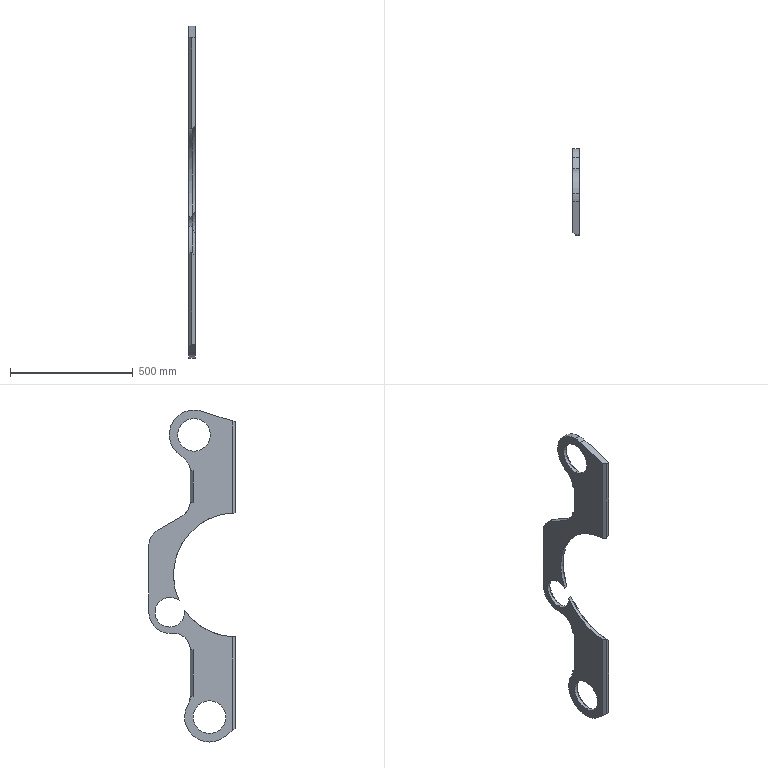Part | SolidWorks | features ICE 3, Chamfer 2, Extrusion 1, Fillet 1 | 1 solid | 46 faces | box 25 x 352.3 x 1354 mm | volume 4602346 mm3 | cylinder 19 | plane 18 | cone 9 | commonest cylinder face diameters 140 x6 133 x4 121 x3 203 x3 506 x2 171 x1
STEP:
#1=CARTESIAN_POINT('',(0.5,169.,637.5));
#2=VERTEX_POINT('',#1);
#3=CARTESIAN_POINT('',(0.5,169.,504.5));
#4=VERTEX_POINT('',#3);
#5=CARTESIAN_POINT('',(0.5,169.,571.));
#6=DIRECTION('',(1.,0.,0.));
#7=DIRECTION('',(0.,0.,-1.));
#8=AXIS2_PLACEMENT_3D('',#5,#6,#7);
#9=CIRCLE('',#8,66.5);
#10=EDGE_CURVE('',#2,#4,#9,.T.);
#11=ORIENTED_EDGE('',*,*,#10,.F.);
#12=CARTESIAN_POINT('',(12.5,169.,649.5));
#13=VERTEX_POINT('',#12);
#14=CARTESIAN_POINT('',(0.5,169.,637.5));
#15=DIRECTION('',(0.7071,0.,0.7071));
#16=VECTOR('',#15,1000.);
#17=LINE('',#14,#16);
#18=EDGE_CURVE('',#2,#13,#17,.T.);
#19=ORIENTED_EDGE('',*,*,#18,.T.);
#20=CARTESIAN_POINT('',(12.5,169.,492.5));
#21=VERTEX_POINT('',#20);
#22=CARTESIAN_POINT('',(12.5,169.,571.));
#23=DIRECTION('',(-1.,0.,0.));
#24=DIRECTION('',(0.,0.,-1.));
#25=AXIS2_PLACEMENT_3D('',#22,#23,#24);
#26=CIRCLE('',#25,78.5);
#27=EDGE_CURVE('',#21,#13,#26,.T.);
#28=ORIENTED_EDGE('',*,*,#27,.F.);
#29=CARTESIAN_POINT('',(0.5,169.,504.5));
#30=DIRECTION('',(0.7071,0.,-0.7071));
#31=VECTOR('',#30,1000.);
#32=LINE('',#29,#31);
#33=EDGE_CURVE('',#4,#21,#32,.T.);
#34=ORIENTED_EDGE('',*,*,#33,.F.);
#35=EDGE_LOOP('',(#11,#19,#28,#34));
#36=FACE_OUTER_BOUND('',#35,.T.);
#37=CARTESIAN_POINT('',(0.5,169.,571.));
#38=DIRECTION('',(1.,0.,0.));
#39=DIRECTION('',(0.,0.,-1.));
#40=AXIS2_PLACEMENT_3D('',#37,#38,#39);
#41=CONICAL_SURFACE('',#40,66.5,0.7854);
#42=ADVANCED_FACE('',(#36),#41,.F.);
#43=CARTESIAN_POINT('',(0.5,268.,-91.9));
#44=VERTEX_POINT('',#43);
#45=CARTESIAN_POINT('',(0.5,230.055,-105.278));
#46=VERTEX_POINT('',#45);
#47=CARTESIAN_POINT('',(0.5,268.,-152.4));
#48=DIRECTION('',(1.,0.,0.));
#49=DIRECTION('',(0.,0.,-1.));
#50=AXIS2_PLACEMENT_3D('',#47,#48,#49);
#51=CIRCLE('',#50,60.5);
#52=EDGE_CURVE('',#44,#46,#51,.T.);
#53=ORIENTED_EDGE('',*,*,#52,.F.);
#54=CARTESIAN_POINT('',(12.5,268.,-79.9));
#55=VERTEX_POINT('',#54);
#56=CARTESIAN_POINT('',(0.5,268.,-91.9));
#57=DIRECTION('',(0.7071,0.,0.7071));
#58=VECTOR('',#57,1000.);
#59=LINE('',#56,#58);
#60=EDGE_CURVE('',#44,#55,#59,.T.);
#61=ORIENTED_EDGE('',*,*,#60,.T.);
#62=CARTESIAN_POINT('',(12.5,252.103,-81.664));
#63=VERTEX_POINT('',#62);
#64=CARTESIAN_POINT('',(12.5,268.,-152.4));
#65=DIRECTION('',(-1.,0.,0.));
#66=DIRECTION('',(0.,0.,-1.));
#67=AXIS2_PLACEMENT_3D('',#64,#65,#66);
#68=CIRCLE('',#67,72.5);
#69=EDGE_CURVE('',#63,#55,#68,.T.);
#70=ORIENTED_EDGE('',*,*,#69,.F.);
#71=CARTESIAN_POINT('',(0.5,230.055,-105.278));
#72=CARTESIAN_POINT('',(1.802,233.534,-100.805));
#73=CARTESIAN_POINT('',(3.525,237.131,-96.657));
#74=CARTESIAN_POINT('',(7.589,244.498,-88.834));
#75=CARTESIAN_POINT('',(9.93,248.268,-85.161));
#76=CARTESIAN_POINT('',(12.5,252.103,-81.664));
#77=B_SPLINE_CURVE_WITH_KNOTS('',3,(#71,#72,#73,#74,#75,#76),.UNSPECIFIED.,.F.,.F.,(4,2,4),(0.,0.01723,0.03446),.UNSPECIFIED.);
#78=EDGE_CURVE('',#46,#63,#77,.T.);
#79=ORIENTED_EDGE('',*,*,#78,.F.);
#80=EDGE_LOOP('',(#53,#61,#70,#79));
#81=FACE_OUTER_BOUND('',#80,.T.);
#82=CARTESIAN_POINT('',(0.5,268.,-152.4));
#83=DIRECTION('',(1.,0.,0.));
#84=DIRECTION('',(0.,0.,-1.));
#85=AXIS2_PLACEMENT_3D('',#82,#83,#84);
#86=CONICAL_SURFACE('',#85,60.5,0.7854);
#87=ADVANCED_FACE('',(#81),#86,.F.);
#88=ORIENTED_EDGE('',*,*,#60,.F.);
#89=CARTESIAN_POINT('',(0.5,268.,-212.9));
#90=VERTEX_POINT('',#89);
#91=CARTESIAN_POINT('',(0.5,268.,-152.4));
#92=DIRECTION('',(1.,0.,0.));
#93=DIRECTION('',(0.,0.,-1.));
#94=AXIS2_PLACEMENT_3D('',#91,#92,#93);
#95=CIRCLE('',#94,60.5);
#96=EDGE_CURVE('',#90,#44,#95,.T.);
#97=ORIENTED_EDGE('',*,*,#96,.F.);
#98=CARTESIAN_POINT('',(12.5,268.,-224.9));
#99=VERTEX_POINT('',#98);
#100=CARTESIAN_POINT('',(0.5,268.,-212.9));
#101=DIRECTION('',(0.7071,0.,-0.7071));
#102=VECTOR('',#101,1000.);
#103=LINE('',#100,#102);
#104=EDGE_CURVE('',#90,#99,#103,.T.);
#105=ORIENTED_EDGE('',*,*,#104,.T.);
#106=CARTESIAN_POINT('',(12.5,268.,-152.4));
#107=DIRECTION('',(-1.,0.,0.));
#108=DIRECTION('',(0.,0.,-1.));
#109=AXIS2_PLACEMENT_3D('',#106,#107,#108);
#110=CIRCLE('',#109,72.5);
#111=EDGE_CURVE('',#55,#99,#110,.T.);
#112=ORIENTED_EDGE('',*,*,#111,.F.);
#113=EDGE_LOOP('',(#88,#97,#105,#112));
#114=FACE_OUTER_BOUND('',#113,.T.);
#115=CARTESIAN_POINT('',(0.5,268.,-152.4));
#116=DIRECTION('',(1.,0.,0.));
#117=DIRECTION('',(0.,0.,-1.));
#118=AXIS2_PLACEMENT_3D('',#115,#116,#117);
#119=CONICAL_SURFACE('',#118,60.5,0.7854);
#120=ADVANCED_FACE('',(#114),#119,.F.);
#121=CARTESIAN_POINT('',(0.5,106.,-513.5));
#122=VERTEX_POINT('',#121);
#123=CARTESIAN_POINT('',(0.5,106.,-646.5));
#124=VERTEX_POINT('',#123);
#125=CARTESIAN_POINT('',(0.5,106.,-580.));
#126=DIRECTION('',(1.,0.,0.));
#127=DIRECTION('',(0.,0.,-1.));
#128=AXIS2_PLACEMENT_3D('',#125,#126,#127);
#129=CIRCLE('',#128,66.5);
#130=EDGE_CURVE('',#122,#124,#129,.T.);
#131=ORIENTED_EDGE('',*,*,#130,.F.);
#132=CARTESIAN_POINT('',(12.5,106.,-501.5));
#133=VERTEX_POINT('',#132);
#134=CARTESIAN_POINT('',(0.5,106.,-513.5));
#135=DIRECTION('',(0.7071,0.,0.7071));
#136=VECTOR('',#135,1000.);
#137=LINE('',#134,#136);
#138=EDGE_CURVE('',#122,#133,#137,.T.);
#139=ORIENTED_EDGE('',*,*,#138,.T.);
#140=CARTESIAN_POINT('',(12.5,106.,-658.5));
#141=VERTEX_POINT('',#140);
#142=CARTESIAN_POINT('',(12.5,106.,-580.));
#143=DIRECTION('',(-1.,0.,0.));
#144=DIRECTION('',(0.,0.,-1.));
#145=AXIS2_PLACEMENT_3D('',#142,#143,#144);
#146=CIRCLE('',#145,78.5);
#147=EDGE_CURVE('',#141,#133,#146,.T.);
#148=ORIENTED_EDGE('',*,*,#147,.F.);
#149=CARTESIAN_POINT('',(0.5,106.,-646.5));
#150=DIRECTION('',(0.7071,0.,-0.7071));
#151=VECTOR('',#150,1000.);
#152=LINE('',#149,#151);
#153=EDGE_CURVE('',#124,#141,#152,.T.);
#154=ORIENTED_EDGE('',*,*,#153,.F.);
#155=EDGE_LOOP('',(#131,#139,#148,#154));
#156=FACE_OUTER_BOUND('',#155,.T.);
#157=CARTESIAN_POINT('',(0.5,106.,-580.));
#158=DIRECTION('',(1.,0.,0.));
#159=DIRECTION('',(0.,0.,-1.));
#160=AXIS2_PLACEMENT_3D('',#157,#158,#159);
#161=CONICAL_SURFACE('',#160,66.5,0.7854);
#162=ADVANCED_FACE('',(#156),#161,.F.);
#163=CARTESIAN_POINT('',(-12.5,106.,-513.5));
#164=VERTEX_POINT('',#163);
#165=CARTESIAN_POINT('',(-12.5,106.,-646.5));
#166=VERTEX_POINT('',#165);
#167=CARTESIAN_POINT('',(-12.5,106.,-580.));
#168=DIRECTION('',(1.,0.,0.));
#169=DIRECTION('',(0.,0.,-1.));
#170=AXIS2_PLACEMENT_3D('',#167,#168,#169);
#171=CIRCLE('',#170,66.5);
#172=EDGE_CURVE('',#164,#166,#171,.T.);
#173=ORIENTED_EDGE('',*,*,#172,.F.);
#174=CARTESIAN_POINT('',(-12.5,106.,-513.5));
#175=DIRECTION('',(1.,0.,0.));
#176=VECTOR('',#175,1000.);
#177=LINE('',#174,#176);
#178=EDGE_CURVE('',#164,#122,#177,.T.);
#179=ORIENTED_EDGE('',*,*,#178,.T.);
#180=ORIENTED_EDGE('',*,*,#130,.T.);
#181=CARTESIAN_POINT('',(-12.5,106.,-646.5));
#182=DIRECTION('',(1.,0.,0.));
#183=VECTOR('',#182,1000.);
#184=LINE('',#181,#183);
#185=EDGE_CURVE('',#166,#124,#184,.T.);
#186=ORIENTED_EDGE('',*,*,#185,.F.);
#187=EDGE_LOOP('',(#173,#179,#180,#186));
#188=FACE_OUTER_BOUND('',#187,.T.);
#189=CARTESIAN_POINT('',(-12.5,106.,-580.));
#190=DIRECTION('',(1.,0.,0.));
#191=DIRECTION('',(0.,0.,-1.));
#192=AXIS2_PLACEMENT_3D('',#189,#190,#191);
#193=CYLINDRICAL_SURFACE('',#192,66.5);
#194=ADVANCED_FACE('',(#188),#193,.F.);
#195=CARTESIAN_POINT('',(-12.5,169.,637.5));
#196=VERTEX_POINT('',#195);
#197=CARTESIAN_POINT('',(-12.5,169.,504.5));
#198=VERTEX_POINT('',#197);
#199=CARTESIAN_POINT('',(-12.5,169.,571.));
#200=DIRECTION('',(1.,0.,0.));
#201=DIRECTION('',(0.,0.,-1.));
#202=AXIS2_PLACEMENT_3D('',#199,#200,#201);
#203=CIRCLE('',#202,66.5);
#204=EDGE_CURVE('',#196,#198,#203,.T.);
#205=ORIENTED_EDGE('',*,*,#204,.F.);
#206=CARTESIAN_POINT('',(-12.5,169.,637.5));
#207=DIRECTION('',(1.,0.,0.));
#208=VECTOR('',#207,1000.);
#209=LINE('',#206,#208);
#210=EDGE_CURVE('',#196,#2,#209,.T.);
#211=ORIENTED_EDGE('',*,*,#210,.T.);
#212=ORIENTED_EDGE('',*,*,#10,.T.);
#213=CARTESIAN_POINT('',(-12.5,169.,504.5));
#214=DIRECTION('',(1.,0.,0.));
#215=VECTOR('',#214,1000.);
#216=LINE('',#213,#215);
#217=EDGE_CURVE('',#198,#4,#216,.T.);
#218=ORIENTED_EDGE('',*,*,#217,.F.);
#219=EDGE_LOOP('',(#205,#211,#212,#218));
#220=FACE_OUTER_BOUND('',#219,.T.);
#221=CARTESIAN_POINT('',(-12.5,169.,571.));
#222=DIRECTION('',(1.,0.,0.));
#223=DIRECTION('',(0.,0.,-1.));
#224=AXIS2_PLACEMENT_3D('',#221,#222,#223);
#225=CYLINDRICAL_SURFACE('',#224,66.5);
#226=ADVANCED_FACE('',(#220),#225,.F.);
#227=CARTESIAN_POINT('',(-12.5,268.,-91.9));
#228=VERTEX_POINT('',#227);
#229=CARTESIAN_POINT('',(-12.5,230.055,-105.278));
#230=VERTEX_POINT('',#229);
#231=CARTESIAN_POINT('',(-12.5,268.,-152.4));
#232=DIRECTION('',(1.,0.,0.));
#233=DIRECTION('',(0.,0.,-1.));
#234=AXIS2_PLACEMENT_3D('',#231,#232,#233);
#235=CIRCLE('',#234,60.5);
#236=EDGE_CURVE('',#228,#230,#235,.T.);
#237=ORIENTED_EDGE('',*,*,#236,.F.);
#238=CARTESIAN_POINT('',(-12.5,268.,-91.9));
#239=DIRECTION('',(1.,0.,0.));
#240=VECTOR('',#239,1000.);
#241=LINE('',#238,#240);
#242=EDGE_CURVE('',#228,#44,#241,.T.);
#243=ORIENTED_EDGE('',*,*,#242,.T.);
#244=ORIENTED_EDGE('',*,*,#52,.T.);
#245=CARTESIAN_POINT('',(0.,230.055,-105.278));
#246=DIRECTION('',(1.,0.,0.));
#247=VECTOR('',#246,1000.);
#248=LINE('',#245,#247);
#249=EDGE_CURVE('',#230,#46,#248,.T.);
#250=ORIENTED_EDGE('',*,*,#249,.F.);
#251=EDGE_LOOP('',(#237,#243,#244,#250));
#252=FACE_OUTER_BOUND('',#251,.T.);
#253=CARTESIAN_POINT('',(-12.5,268.,-152.4));
#254=DIRECTION('',(1.,0.,0.));
#255=DIRECTION('',(0.,0.,-1.));
#256=AXIS2_PLACEMENT_3D('',#253,#254,#255);
#257=CYLINDRICAL_SURFACE('',#256,60.5);
#258=ADVANCED_FACE('',(#252),#257,.F.);
#259=ORIENTED_EDGE('',*,*,#242,.F.);
#260=CARTESIAN_POINT('',(-12.5,268.,-212.9));
#261=VERTEX_POINT('',#260);
#262=CARTESIAN_POINT('',(-12.5,268.,-152.4));
#263=DIRECTION('',(1.,0.,0.));
#264=DIRECTION('',(0.,0.,-1.));
#265=AXIS2_PLACEMENT_3D('',#262,#263,#264);
#266=CIRCLE('',#265,60.5);
#267=EDGE_CURVE('',#261,#228,#266,.T.);
#268=ORIENTED_EDGE('',*,*,#267,.F.);
#269=CARTESIAN_POINT('',(-12.5,268.,-212.9));
#270=DIRECTION('',(1.,0.,0.));
#271=VECTOR('',#270,1000.);
#272=LINE('',#269,#271);
#273=EDGE_CURVE('',#261,#90,#272,.T.);
#274=ORIENTED_EDGE('',*,*,#273,.T.);
#275=ORIENTED_EDGE('',*,*,#96,.T.);
#276=EDGE_LOOP('',(#259,#268,#274,#275));
#277=FACE_OUTER_BOUND('',#276,.T.);
#278=CARTESIAN_POINT('',(-12.5,268.,-152.4));
#279=DIRECTION('',(1.,0.,0.));
#280=DIRECTION('',(0.,0.,-1.));
#281=AXIS2_PLACEMENT_3D('',#278,#279,#280);
#282=CYLINDRICAL_SURFACE('',#281,60.5);
#283=ADVANCED_FACE('',(#277),#282,.F.);
#284=CARTESIAN_POINT('',(12.5,254.,-237.268));
#285=VERTEX_POINT('',#284);
#286=CARTESIAN_POINT('',(12.5,260.302,-237.553));
#287=VERTEX_POINT('',#286);
#288=CARTESIAN_POINT('',(12.5,254.,-307.268));
#289=DIRECTION('',(-1.,0.,0.));
#290=DIRECTION('',(0.,0.,-1.));
#291=AXIS2_PLACEMENT_3D('',#288,#289,#290);
#292=CIRCLE('',#291,70.);
#293=EDGE_CURVE('',#285,#287,#292,.T.);
#294=ORIENTED_EDGE('',*,*,#293,.F.);
#295=CARTESIAN_POINT('',(-12.5,254.,-237.268));
#296=VERTEX_POINT('',#295);
#297=CARTESIAN_POINT('',(12.5,254.,-237.268));
#298=DIRECTION('',(-1.,0.,0.));
#299=VECTOR('',#298,1000.);
#300=LINE('',#297,#299);
#301=EDGE_CURVE('',#285,#296,#300,.T.);
#302=ORIENTED_EDGE('',*,*,#301,.T.);
#303=CARTESIAN_POINT('',(-12.5,260.302,-237.553));
#304=VERTEX_POINT('',#303);
#305=CARTESIAN_POINT('',(-12.5,254.,-307.268));
#306=DIRECTION('',(-1.,0.,0.));
#307=DIRECTION('',(0.,0.,-1.));
#308=AXIS2_PLACEMENT_3D('',#305,#306,#307);
#309=CIRCLE('',#308,70.);
#310=EDGE_CURVE('',#296,#304,#309,.T.);
#311=ORIENTED_EDGE('',*,*,#310,.T.);
#312=CARTESIAN_POINT('',(12.5,260.302,-237.553));
#313=DIRECTION('',(-1.,0.,0.));
#314=VECTOR('',#313,1000.);
#315=LINE('',#312,#314);
#316=EDGE_CURVE('',#287,#304,#315,.T.);
#317=ORIENTED_EDGE('',*,*,#316,.F.);
#318=EDGE_LOOP('',(#294,#302,#311,#317));
#319=FACE_OUTER_BOUND('',#318,.T.);
#320=CARTESIAN_POINT('',(12.5,254.,-307.268));
#321=DIRECTION('',(-1.,0.,0.));
#322=DIRECTION('',(0.,0.,1.));
#323=AXIS2_PLACEMENT_3D('',#320,#321,#322);
#324=CYLINDRICAL_SURFACE('',#323,70.);
#325=ADVANCED_FACE('',(#319),#324,.F.);
#326=CARTESIAN_POINT('',(12.5,169.,672.5));
#327=VERTEX_POINT('',#326);
#328=CARTESIAN_POINT('',(12.5,138.146,667.697));
#329=VERTEX_POINT('',#328);
#330=CARTESIAN_POINT('',(12.5,169.,571.));
#331=DIRECTION('',(1.,0.,0.));
#332=DIRECTION('',(0.,0.,-1.));
#333=AXIS2_PLACEMENT_3D('',#330,#331,#332);
#334=CIRCLE('',#333,101.5);
#335=EDGE_CURVE('',#327,#329,#334,.T.);
#336=ORIENTED_EDGE('',*,*,#335,.F.);
#337=CARTESIAN_POINT('',(-12.5,169.,672.5));
#338=VERTEX_POINT('',#337);
#339=CARTESIAN_POINT('',(12.5,169.,672.5));
#340=DIRECTION('',(-1.,0.,0.));
#341=VECTOR('',#340,1000.);
#342=LINE('',#339,#341);
#343=EDGE_CURVE('',#327,#338,#342,.T.);
#344=ORIENTED_EDGE('',*,*,#343,.T.);
#345=CARTESIAN_POINT('',(-12.5,138.146,667.697));
#346=VERTEX_POINT('',#345);
#347=CARTESIAN_POINT('',(-12.5,169.,571.));
#348=DIRECTION('',(1.,0.,0.));
#349=DIRECTION('',(0.,0.,-1.));
#350=AXIS2_PLACEMENT_3D('',#347,#348,#349);
#351=CIRCLE('',#350,101.5);
#352=EDGE_CURVE('',#338,#346,#351,.T.);
#353=ORIENTED_EDGE('',*,*,#352,.T.);
#354=CARTESIAN_POINT('',(12.5,138.146,667.697));
#355=DIRECTION('',(-1.,0.,0.));
#356=VECTOR('',#355,1000.);
#357=LINE('',#354,#356);
#358=EDGE_CURVE('',#329,#346,#357,.T.);
#359=ORIENTED_EDGE('',*,*,#358,.F.);
#360=EDGE_LOOP('',(#336,#344,#353,#359));
#361=FACE_OUTER_BOUND('',#360,.T.);
#362=CARTESIAN_POINT('',(12.5,169.,571.));
#363=DIRECTION('',(-1.,0.,0.));
#364=DIRECTION('',(0.,0.,1.));
#365=AXIS2_PLACEMENT_3D('',#362,#363,#364);
#366=CYLINDRICAL_SURFACE('',#365,101.5);
#367=ADVANCED_FACE('',(#361),#366,.T.);
#368=CARTESIAN_POINT('',(-12.5,106.,-580.));
#369=DIRECTION('',(1.,0.,0.));
#370=DIRECTION('',(0.,0.,-1.));
#371=AXIS2_PLACEMENT_3D('',#368,#369,#370);
#372=CIRCLE('',#371,66.5);
#373=EDGE_CURVE('',#166,#164,#372,.T.);
#374=ORIENTED_EDGE('',*,*,#373,.T.);
#375=ORIENTED_EDGE('',*,*,#172,.T.);
#376=EDGE_LOOP('',(#374,#375));
#377=FACE_BOUND('',#376,.T.);
#378=CARTESIAN_POINT('',(-12.5,169.,571.));
#379=DIRECTION('',(1.,0.,0.));
#380=DIRECTION('',(0.,0.,-1.));
#381=AXIS2_PLACEMENT_3D('',#378,#379,#380);
#382=CIRCLE('',#381,66.5);
#383=EDGE_CURVE('',#198,#196,#382,.T.);
#384=ORIENTED_EDGE('',*,*,#383,.T.);
#385=ORIENTED_EDGE('',*,*,#204,.T.);
#386=EDGE_LOOP('',(#384,#385));
#387=FACE_BOUND('',#386,.T.);
#388=CARTESIAN_POINT('',(-12.5,184.019,-495.));
#389=VERTEX_POINT('',#388);
#390=CARTESIAN_POINT('',(-12.5,172.,-495.));
#391=VERTEX_POINT('',#390);
#392=CARTESIAN_POINT('',(-12.5,190.,-495.));
#393=DIRECTION('',(0.,-1.,0.));
#394=VECTOR('',#393,1000.);
#395=LINE('',#392,#394);
#396=EDGE_CURVE('',#389,#391,#395,.T.);
#397=ORIENTED_EDGE('',*,*,#396,.F.);
#398=CARTESIAN_POINT('',(-12.5,193.592,-528.717));
#399=VERTEX_POINT('',#398);
#400=CARTESIAN_POINT('',(-12.5,254.,-493.35));
#401=DIRECTION('',(1.,0.,0.));
#402=DIRECTION('',(0.,0.,-1.));
#403=AXIS2_PLACEMENT_3D('',#400,#401,#402);
#404=CIRCLE('',#403,70.);
#405=EDGE_CURVE('',#389,#399,#404,.T.);
#406=ORIENTED_EDGE('',*,*,#405,.T.);
#407=CARTESIAN_POINT('',(-12.5,40.757,-657.754));
#408=VERTEX_POINT('',#407);
#409=CARTESIAN_POINT('',(-12.5,106.,-580.));
#410=DIRECTION('',(1.,0.,0.));
#411=DIRECTION('',(0.,0.,-1.));
#412=AXIS2_PLACEMENT_3D('',#409,#410,#411);
#413=CIRCLE('',#412,101.5);
#414=EDGE_CURVE('',#408,#399,#413,.T.);
#415=ORIENTED_EDGE('',*,*,#414,.F.);
#416=CARTESIAN_POINT('',(-12.5,13.2,-634.63));
#417=VERTEX_POINT('',#416);
#418=CARTESIAN_POINT('',(-12.5,40.757,-657.754));
#419=DIRECTION('',(0.,0.766,-0.6428));
#420=VECTOR('',#419,1000.);
#421=LINE('',#418,#420);
#422=EDGE_CURVE('',#417,#408,#421,.T.);
#423=ORIENTED_EDGE('',*,*,#422,.F.);
#424=CARTESIAN_POINT('',(-12.5,13.2,-252.655));
#425=VERTEX_POINT('',#424);
#426=CARTESIAN_POINT('',(-12.5,13.2,571.));
#427=DIRECTION('',(0.,0.,1.));
#428=VECTOR('',#427,1000.);
#429=LINE('',#426,#428);
#430=EDGE_CURVE('',#417,#425,#429,.T.);
#431=ORIENTED_EDGE('',*,*,#430,.T.);
#432=CARTESIAN_POINT('',(-12.5,208.102,-143.883));
#433=VERTEX_POINT('',#432);
#434=CARTESIAN_POINT('',(-12.5,0.,0.));
#435=DIRECTION('',(-1.,0.,0.));
#436=DIRECTION('',(0.,0.,-1.));
#437=AXIS2_PLACEMENT_3D('',#434,#435,#436);
#438=CIRCLE('',#437,253.);
#439=EDGE_CURVE('',#433,#425,#438,.T.);
#440=ORIENTED_EDGE('',*,*,#439,.F.);
#441=CARTESIAN_POINT('',(-12.5,268.,-152.4));
#442=DIRECTION('',(1.,0.,0.));
#443=DIRECTION('',(0.,0.,-1.));
#444=AXIS2_PLACEMENT_3D('',#441,#442,#443);
#445=CIRCLE('',#444,60.5);
#446=EDGE_CURVE('',#433,#261,#445,.T.);
#447=ORIENTED_EDGE('',*,*,#446,.T.);
#448=ORIENTED_EDGE('',*,*,#267,.T.);
#449=ORIENTED_EDGE('',*,*,#236,.T.);
#450=CARTESIAN_POINT('',(-12.5,13.2,252.655));
#451=VERTEX_POINT('',#450);
#452=CARTESIAN_POINT('',(-12.5,0.,0.));
#453=DIRECTION('',(-1.,0.,0.));
#454=DIRECTION('',(0.,0.,-1.));
#455=AXIS2_PLACEMENT_3D('',#452,#453,#454);
#456=CIRCLE('',#455,253.);
#457=EDGE_CURVE('',#451,#230,#456,.T.);
#458=ORIENTED_EDGE('',*,*,#457,.F.);
#459=CARTESIAN_POINT('',(-12.5,13.2,627.829));
#460=VERTEX_POINT('',#459);
#461=CARTESIAN_POINT('',(-12.5,13.2,571.));
#462=DIRECTION('',(0.,0.,1.));
#463=VECTOR('',#462,1000.);
#464=LINE('',#461,#463);
#465=EDGE_CURVE('',#451,#460,#464,.T.);
#466=ORIENTED_EDGE('',*,*,#465,.T.);
#467=CARTESIAN_POINT('',(-12.5,1.2,624.));
#468=DIRECTION('',(0.,-0.9527,-0.304));
#469=VECTOR('',#468,1000.);
#470=LINE('',#467,#469);
#471=EDGE_CURVE('',#346,#460,#470,.T.);
#472=ORIENTED_EDGE('',*,*,#471,.F.);
#473=ORIENTED_EDGE('',*,*,#352,.F.);
#474=CARTESIAN_POINT('',(-12.5,219.306,482.844));
#475=VERTEX_POINT('',#474);
#476=CARTESIAN_POINT('',(-12.5,169.,571.));
#477=DIRECTION('',(1.,0.,0.));
#478=DIRECTION('',(0.,0.,-1.));
#479=AXIS2_PLACEMENT_3D('',#476,#477,#478);
#480=CIRCLE('',#479,101.5);
#481=EDGE_CURVE('',#475,#338,#480,.T.);
#482=ORIENTED_EDGE('',*,*,#481,.F.);
#483=CARTESIAN_POINT('',(-12.5,184.062,425.));
#484=VERTEX_POINT('',#483);
#485=CARTESIAN_POINT('',(-12.5,254.,422.046));
#486=DIRECTION('',(1.,0.,0.));
#487=DIRECTION('',(0.,0.,-1.));
#488=AXIS2_PLACEMENT_3D('',#485,#486,#487);
#489=CIRCLE('',#488,70.);
#490=EDGE_CURVE('',#475,#484,#489,.T.);
#491=ORIENTED_EDGE('',*,*,#490,.T.);
#492=CARTESIAN_POINT('',(-12.5,172.,425.));
#493=VERTEX_POINT('',#492);
#494=CARTESIAN_POINT('',(-12.5,172.,425.));
#495=DIRECTION('',(0.,-1.,0.));
#496=VECTOR('',#495,1000.);
#497=LINE('',#494,#496);
#498=EDGE_CURVE('',#484,#493,#497,.T.);
#499=ORIENTED_EDGE('',*,*,#498,.T.);
#500=CARTESIAN_POINT('',(-12.5,172.,295.));
#501=VERTEX_POINT('',#500);
#502=CARTESIAN_POINT('',(-12.5,172.,295.));
#503=DIRECTION('',(0.,0.,1.));
#504=VECTOR('',#503,1000.);
#505=LINE('',#502,#504);
#506=EDGE_CURVE('',#501,#493,#505,.T.);
#507=ORIENTED_EDGE('',*,*,#506,.F.);
#508=CARTESIAN_POINT('',(-12.5,184.139,295.));
#509=VERTEX_POINT('',#508);
#510=CARTESIAN_POINT('',(-12.5,172.,295.));
#511=DIRECTION('',(0.,-1.,0.));
#512=VECTOR('',#511,1000.);
#513=LINE('',#510,#512);
#514=EDGE_CURVE('',#509,#501,#513,.T.);
#515=ORIENTED_EDGE('',*,*,#514,.F.);
#516=CARTESIAN_POINT('',(-12.5,219.,238.793));
#517=VERTEX_POINT('',#516);
#518=CARTESIAN_POINT('',(-12.5,254.,299.415));
#519=DIRECTION('',(1.,0.,0.));
#520=DIRECTION('',(0.,0.,-1.));
#521=AXIS2_PLACEMENT_3D('',#518,#519,#520);
#522=CIRCLE('',#521,70.);
#523=EDGE_CURVE('',#509,#517,#522,.T.);
#524=ORIENTED_EDGE('',*,*,#523,.T.);
#525=CARTESIAN_POINT('',(-12.5,318.5,181.346));
#526=VERTEX_POINT('',#525);
#527=CARTESIAN_POINT('',(-12.5,353.5,161.139));
#528=DIRECTION('',(0.,-0.866,0.5));
#529=VECTOR('',#528,1000.);
#530=LINE('',#527,#529);
#531=EDGE_CURVE('',#526,#517,#530,.T.);
#532=ORIENTED_EDGE('',*,*,#531,.F.);
#533=CARTESIAN_POINT('',(-12.5,353.5,120.725));
#534=VERTEX_POINT('',#533);
#535=CARTESIAN_POINT('',(-12.5,283.5,120.725));
#536=DIRECTION('',(-1.,0.,0.));
#537=DIRECTION('',(0.,0.,-1.));
#538=AXIS2_PLACEMENT_3D('',#535,#536,#537);
#539=CIRCLE('',#538,70.);
#540=EDGE_CURVE('',#526,#534,#539,.T.);
#541=ORIENTED_EDGE('',*,*,#540,.T.);
#542=CARTESIAN_POINT('',(-12.5,353.5,-152.4));
#543=VERTEX_POINT('',#542);
#544=CARTESIAN_POINT('',(-12.5,353.5,161.139));
#545=DIRECTION('',(0.,0.,1.));
#546=VECTOR('',#545,1000.);
#547=LINE('',#544,#546);
#548=EDGE_CURVE('',#543,#534,#547,.T.);
#549=ORIENTED_EDGE('',*,*,#548,.F.);
#550=CARTESIAN_POINT('',(-12.5,268.,-152.4));
#551=DIRECTION('',(1.,0.,0.));
#552=DIRECTION('',(0.,0.,-1.));
#553=AXIS2_PLACEMENT_3D('',#550,#551,#552);
#554=CIRCLE('',#553,85.5);
#555=EDGE_CURVE('',#304,#543,#554,.T.);
#556=ORIENTED_EDGE('',*,*,#555,.F.);
#557=ORIENTED_EDGE('',*,*,#310,.F.);
#558=CARTESIAN_POINT('',(-12.5,184.037,-305.));
#559=VERTEX_POINT('',#558);
#560=CARTESIAN_POINT('',(-12.5,254.,-307.268));
#561=DIRECTION('',(-1.,0.,0.));
#562=DIRECTION('',(0.,0.,-1.));
#563=AXIS2_PLACEMENT_3D('',#560,#561,#562);
#564=CIRCLE('',#563,70.);
#565=EDGE_CURVE('',#559,#296,#564,.T.);
#566=ORIENTED_EDGE('',*,*,#565,.F.);
#567=CARTESIAN_POINT('',(-12.5,172.,-305.));
#568=VERTEX_POINT('',#567);
#569=CARTESIAN_POINT('',(-12.5,190.,-305.));
#570=DIRECTION('',(0.,-1.,0.));
#571=VECTOR('',#570,1000.);
#572=LINE('',#569,#571);
#573=EDGE_CURVE('',#559,#568,#572,.T.);
#574=ORIENTED_EDGE('',*,*,#573,.T.);
#575=CARTESIAN_POINT('',(-12.5,172.,-495.));
#576=DIRECTION('',(0.,0.,1.));
#577=VECTOR('',#576,1000.);
#578=LINE('',#575,#577);
#579=EDGE_CURVE('',#391,#568,#578,.T.);
#580=ORIENTED_EDGE('',*,*,#579,.F.);
#581=EDGE_LOOP('',(#397,#406,#415,#423,#431,#440,#447,#448,#449,#458,#466,#472,#473,#482,#491,#499,#507,#515,#524,#532,#541,#549,#556,#557,#566,#574,#580));
#582=FACE_OUTER_BOUND('',#581,.T.);
#583=CARTESIAN_POINT('',(-12.5,169.,571.));
#584=DIRECTION('',(1.,0.,0.));
#585=DIRECTION('',(0.,0.,-1.));
#586=AXIS2_PLACEMENT_3D('',#583,#584,#585);
#587=PLANE('',#586);
#588=ADVANCED_FACE('',(#377,#387,#582),#587,.F.);
#589=ORIENTED_EDGE('',*,*,#439,.T.);
#590=CARTESIAN_POINT('',(-0.5,1.2,-252.997));
#591=VERTEX_POINT('',#590);
#592=CARTESIAN_POINT('',(-12.5,13.2,-252.655));
#593=CARTESIAN_POINT('',(-8.503,9.203,-252.864));
#594=CARTESIAN_POINT('',(-4.502,5.202,-252.978));
#595=CARTESIAN_POINT('',(-0.5,1.2,-252.997));
#596=(BOUNDED_CURVE()B_SPLINE_CURVE(3,(#592,#593,#594,#595),.UNSPECIFIED.,.F.,.T.)B_SPLINE_CURVE_WITH_KNOTS((4,4),(1.519,1.566),.UNSPECIFIED.)CURVE()GEOMETRIC_REPRESENTATION_ITEM()RATIONAL_B_SPLINE_CURVE((1.,0.9998,0.9998,1.))REPRESENTATION_ITEM(''));
#597=EDGE_CURVE('',#425,#591,#596,.T.);
#598=ORIENTED_EDGE('',*,*,#597,.T.);
#599=CARTESIAN_POINT('',(0.5,1.2,-252.997));
#600=VERTEX_POINT('',#599);
#601=CARTESIAN_POINT('',(12.5,1.2,-252.997));
#602=DIRECTION('',(-1.,0.,0.));
#603=VECTOR('',#602,1000.);
#604=LINE('',#601,#603);
#605=EDGE_CURVE('',#600,#591,#604,.T.);
#606=ORIENTED_EDGE('',*,*,#605,.F.);
#607=CARTESIAN_POINT('',(0.5,208.102,-143.883));
#608=VERTEX_POINT('',#607);
#609=CARTESIAN_POINT('',(0.5,0.,0.));
#610=DIRECTION('',(1.,0.,0.));
#611=DIRECTION('',(0.,0.,-1.));
#612=AXIS2_PLACEMENT_3D('',#609,#610,#611);
#613=CIRCLE('',#612,253.);
#614=EDGE_CURVE('',#600,#608,#613,.T.);
#615=ORIENTED_EDGE('',*,*,#614,.T.);
#616=CARTESIAN_POINT('',(0.,208.102,-143.883));
#617=DIRECTION('',(-1.,0.,0.));
#618=VECTOR('',#617,1000.);
#619=LINE('',#616,#618);
#620=EDGE_CURVE('',#608,#433,#619,.T.);
#621=ORIENTED_EDGE('',*,*,#620,.T.);
#622=EDGE_LOOP('',(#589,#598,#606,#615,#621));
#623=FACE_OUTER_BOUND('',#622,.T.);
#624=CARTESIAN_POINT('',(12.5,0.,0.));
#625=DIRECTION('',(-1.,0.,0.));
#626=DIRECTION('',(0.,0.,1.));
#627=AXIS2_PLACEMENT_3D('',#624,#625,#626);
#628=CYLINDRICAL_SURFACE('',#627,253.);
#629=ADVANCED_FACE('',(#623),#628,.F.);
#630=ORIENTED_EDGE('',*,*,#343,.F.);
#631=CARTESIAN_POINT('',(12.5,219.306,482.844));
#632=VERTEX_POINT('',#631);
#633=CARTESIAN_POINT('',(12.5,169.,571.));
#634=DIRECTION('',(1.,0.,0.));
#635=DIRECTION('',(0.,0.,-1.));
#636=AXIS2_PLACEMENT_3D('',#633,#634,#635);
#637=CIRCLE('',#636,101.5);
#638=EDGE_CURVE('',#632,#327,#637,.T.);
#639=ORIENTED_EDGE('',*,*,#638,.F.);
#640=CARTESIAN_POINT('',(12.5,219.306,482.844));
#641=DIRECTION('',(-1.,0.,0.));
#642=VECTOR('',#641,1000.);
#643=LINE('',#640,#642);
#644=EDGE_CURVE('',#632,#475,#643,.T.);
#645=ORIENTED_EDGE('',*,*,#644,.T.);
#646=ORIENTED_EDGE('',*,*,#481,.T.);
#647=EDGE_LOOP('',(#630,#639,#645,#646));
#648=FACE_OUTER_BOUND('',#647,.T.);
#649=CARTESIAN_POINT('',(12.5,169.,571.));
#650=DIRECTION('',(-1.,0.,0.));
#651=DIRECTION('',(0.,0.,1.));
#652=AXIS2_PLACEMENT_3D('',#649,#650,#651);
#653=CYLINDRICAL_SURFACE('',#652,101.5);
#654=ADVANCED_FACE('',(#648),#653,.T.);
#655=ORIENTED_EDGE('',*,*,#471,.T.);
#656=CARTESIAN_POINT('',(-0.5,1.2,624.));
#657=VERTEX_POINT('',#656);
#658=CARTESIAN_POINT('',(-0.5,1.2,624.));
#659=DIRECTION('',(0.6898,-0.6898,-0.2201));
#660=VECTOR('',#659,1000.);
#661=LINE('',#658,#660);
#662=EDGE_CURVE('',#460,#657,#661,.T.);
#663=ORIENTED_EDGE('',*,*,#662,.T.);
#664=CARTESIAN_POINT('',(12.5,1.2,624.));
#665=VERTEX_POINT('',#664);
#666=CARTESIAN_POINT('',(12.5,1.2,624.));
#667=DIRECTION('',(-1.,0.,0.));
#668=VECTOR('',#667,1000.);
#669=LINE('',#666,#668);
#670=EDGE_CURVE('',#665,#657,#669,.T.);
#671=ORIENTED_EDGE('',*,*,#670,.F.);
#672=CARTESIAN_POINT('',(12.5,1.2,624.));
#673=DIRECTION('',(0.,-0.9527,-0.304));
#674=VECTOR('',#673,1000.);
#675=LINE('',#672,#674);
#676=EDGE_CURVE('',#329,#665,#675,.T.);
#677=ORIENTED_EDGE('',*,*,#676,.F.);
#678=ORIENTED_EDGE('',*,*,#358,.T.);
#679=EDGE_LOOP('',(#655,#663,#671,#677,#678));
#680=FACE_OUTER_BOUND('',#679,.T.);
#681=CARTESIAN_POINT('',(12.5,1.2,624.));
#682=DIRECTION('',(0.,0.304,-0.9527));
#683=DIRECTION('',(0.,0.9527,0.304));
#684=AXIS2_PLACEMENT_3D('',#681,#682,#683);
#685=PLANE('',#684);
#686=ADVANCED_FACE('',(#680),#685,.F.);
#687=ORIENTED_EDGE('',*,*,#670,.T.);
#688=CARTESIAN_POINT('',(-0.5,1.2,252.997));
#689=VERTEX_POINT('',#688);
#690=CARTESIAN_POINT('',(-0.5,1.2,624.));
#691=DIRECTION('',(0.,0.,-1.));
#692=VECTOR('',#691,1000.);
#693=LINE('',#690,#692);
#694=EDGE_CURVE('',#657,#689,#693,.T.);
#695=ORIENTED_EDGE('',*,*,#694,.T.);
#696=CARTESIAN_POINT('',(0.5,1.2,252.997));
#697=VERTEX_POINT('',#696);
#698=CARTESIAN_POINT('',(12.5,1.2,252.997));
#699=DIRECTION('',(-1.,0.,0.));
#700=VECTOR('',#699,1000.);
#701=LINE('',#698,#700);
#702=EDGE_CURVE('',#697,#689,#701,.T.);
#703=ORIENTED_EDGE('',*,*,#702,.F.);
#704=CARTESIAN_POINT('',(12.5,1.2,264.997));
#705=VERTEX_POINT('',#704);
#706=CARTESIAN_POINT('',(0.5,1.2,252.997));
#707=CARTESIAN_POINT('',(4.5,1.2,256.997));
#708=CARTESIAN_POINT('',(8.5,1.2,260.997));
#709=CARTESIAN_POINT('',(12.5,1.2,264.997));
#710=B_SPLINE_CURVE_WITH_KNOTS('',3,(#706,#707,#708,#709),.UNSPECIFIED.,.F.,.F.,(4,4),(0.,0.01697),.UNSPECIFIED.);
#711=EDGE_CURVE('',#697,#705,#710,.T.);
#712=ORIENTED_EDGE('',*,*,#711,.T.);
#713=CARTESIAN_POINT('',(12.5,1.2,624.));
#714=DIRECTION('',(0.,0.,-1.));
#715=VECTOR('',#714,1000.);
#716=LINE('',#713,#715);
#717=EDGE_CURVE('',#665,#705,#716,.T.);
#718=ORIENTED_EDGE('',*,*,#717,.F.);
#719=EDGE_LOOP('',(#687,#695,#703,#712,#718));
#720=FACE_OUTER_BOUND('',#719,.T.);
#721=CARTESIAN_POINT('',(12.5,1.2,624.));
#722=DIRECTION('',(0.,1.,0.));
#723=DIRECTION('',(0.,0.,1.));
#724=AXIS2_PLACEMENT_3D('',#721,#722,#723);
#725=PLANE('',#724);
#726=ADVANCED_FACE('',(#720),#725,.F.);
#727=ORIENTED_EDGE('',*,*,#702,.T.);
#728=CARTESIAN_POINT('',(-0.5,1.2,252.997));
#729=CARTESIAN_POINT('',(-4.502,5.202,252.978));
#730=CARTESIAN_POINT('',(-8.503,9.203,252.864));
#731=CARTESIAN_POINT('',(-12.5,13.2,252.655));
#732=(BOUNDED_CURVE()B_SPLINE_CURVE(3,(#728,#729,#730,#731),.UNSPECIFIED.,.F.,.F.)B_SPLINE_CURVE_WITH_KNOTS((4,4),(4.717,4.765),.UNSPECIFIED.)CURVE()GEOMETRIC_REPRESENTATION_ITEM()RATIONAL_B_SPLINE_CURVE((1.,0.9998,0.9998,1.))REPRESENTATION_ITEM(''));
#733=EDGE_CURVE('',#689,#451,#732,.T.);
#734=ORIENTED_EDGE('',*,*,#733,.T.);
#735=ORIENTED_EDGE('',*,*,#457,.T.);
#736=ORIENTED_EDGE('',*,*,#249,.T.);
#737=CARTESIAN_POINT('',(0.5,0.,0.));
#738=DIRECTION('',(1.,0.,0.));
#739=DIRECTION('',(0.,0.,-1.));
#740=AXIS2_PLACEMENT_3D('',#737,#738,#739);
#741=CIRCLE('',#740,253.);
#742=EDGE_CURVE('',#46,#697,#741,.T.);
#743=ORIENTED_EDGE('',*,*,#742,.T.);
#744=EDGE_LOOP('',(#727,#734,#735,#736,#743));
#745=FACE_OUTER_BOUND('',#744,.T.);
#746=CARTESIAN_POINT('',(12.5,0.,0.));
#747=DIRECTION('',(-1.,0.,0.));
#748=DIRECTION('',(0.,0.,1.));
#749=AXIS2_PLACEMENT_3D('',#746,#747,#748);
#750=CYLINDRICAL_SURFACE('',#749,253.);
#751=ADVANCED_FACE('',(#745),#750,.F.);
#752=ORIENTED_EDGE('',*,*,#605,.T.);
#753=CARTESIAN_POINT('',(-0.5,1.2,-624.561));
#754=VERTEX_POINT('',#753);
#755=CARTESIAN_POINT('',(-0.5,1.2,-624.561));
#756=DIRECTION('',(0.,0.,-1.));
#757=VECTOR('',#756,1000.);
#758=LINE('',#755,#757);
#759=EDGE_CURVE('',#591,#754,#758,.T.);
#760=ORIENTED_EDGE('',*,*,#759,.T.);
#761=CARTESIAN_POINT('',(12.5,1.2,-624.561));
#762=VERTEX_POINT('',#761);
#763=CARTESIAN_POINT('',(12.5,1.2,-624.561));
#764=DIRECTION('',(-1.,0.,0.));
#765=VECTOR('',#764,1000.);
#766=LINE('',#763,#765);
#767=EDGE_CURVE('',#762,#754,#766,.T.);
#768=ORIENTED_EDGE('',*,*,#767,.F.);
#769=CARTESIAN_POINT('',(12.5,1.2,-264.997));
#770=VERTEX_POINT('',#769);
#771=CARTESIAN_POINT('',(12.5,1.2,-624.561));
#772=DIRECTION('',(0.,0.,-1.));
#773=VECTOR('',#772,1000.);
#774=LINE('',#771,#773);
#775=EDGE_CURVE('',#770,#762,#774,.T.);
#776=ORIENTED_EDGE('',*,*,#775,.F.);
#777=CARTESIAN_POINT('',(12.5,1.2,-264.997));
#778=CARTESIAN_POINT('',(8.5,1.2,-260.997));
#779=CARTESIAN_POINT('',(4.5,1.2,-256.997));
#780=CARTESIAN_POINT('',(0.5,1.2,-252.997));
#781=B_SPLINE_CURVE_WITH_KNOTS('',3,(#777,#778,#779,#780),.UNSPECIFIED.,.F.,.F.,(4,4),(0.,0.01697),.UNSPECIFIED.);
#782=EDGE_CURVE('',#770,#600,#781,.T.);
#783=ORIENTED_EDGE('',*,*,#782,.T.);
#784=EDGE_LOOP('',(#752,#760,#768,#776,#783));
#785=FACE_OUTER_BOUND('',#784,.T.);
#786=CARTESIAN_POINT('',(12.5,1.2,-624.561));
#787=DIRECTION('',(0.,1.,0.));
#788=DIRECTION('',(0.,0.,1.));
#789=AXIS2_PLACEMENT_3D('',#786,#787,#788);
#790=PLANE('',#789);
#791=ADVANCED_FACE('',(#785),#790,.F.);
#792=ORIENTED_EDGE('',*,*,#767,.T.);
#793=CARTESIAN_POINT('',(-0.5,1.2,-624.561));
#794=DIRECTION('',(-0.6081,0.6081,-0.5103));
#795=VECTOR('',#794,1000.);
#796=LINE('',#793,#795);
#797=EDGE_CURVE('',#754,#417,#796,.T.);
#798=ORIENTED_EDGE('',*,*,#797,.T.);
#799=ORIENTED_EDGE('',*,*,#422,.T.);
#800=CARTESIAN_POINT('',(12.5,40.757,-657.754));
#801=VERTEX_POINT('',#800);
#802=CARTESIAN_POINT('',(12.5,40.757,-657.754));
#803=DIRECTION('',(-1.,0.,0.));
#804=VECTOR('',#803,1000.);
#805=LINE('',#802,#804);
#806=EDGE_CURVE('',#801,#408,#805,.T.);
#807=ORIENTED_EDGE('',*,*,#806,.F.);
#808=CARTESIAN_POINT('',(12.5,40.757,-657.754));
#809=DIRECTION('',(0.,0.766,-0.6428));
#810=VECTOR('',#809,1000.);
#811=LINE('',#808,#810);
#812=EDGE_CURVE('',#762,#801,#811,.T.);
#813=ORIENTED_EDGE('',*,*,#812,.F.);
#814=EDGE_LOOP('',(#792,#798,#799,#807,#813));
#815=FACE_OUTER_BOUND('',#814,.T.);
#816=CARTESIAN_POINT('',(12.5,40.757,-657.754));
#817=DIRECTION('',(0.,0.6428,0.766));
#818=DIRECTION('',(0.,-0.766,0.6428));
#819=AXIS2_PLACEMENT_3D('',#816,#817,#818);
#820=PLANE('',#819);
#821=ADVANCED_FACE('',(#815),#820,.F.);
#822=ORIENTED_EDGE('',*,*,#414,.T.);
#823=CARTESIAN_POINT('',(12.5,193.592,-528.717));
#824=VERTEX_POINT('',#823);
#825=CARTESIAN_POINT('',(12.5,193.592,-528.717));
#826=DIRECTION('',(1.,0.,0.));
#827=VECTOR('',#826,1000.);
#828=LINE('',#825,#827);
#829=EDGE_CURVE('',#399,#824,#828,.T.);
#830=ORIENTED_EDGE('',*,*,#829,.T.);
#831=CARTESIAN_POINT('',(12.5,106.,-580.));
#832=DIRECTION('',(1.,0.,0.));
#833=DIRECTION('',(0.,0.,-1.));
#834=AXIS2_PLACEMENT_3D('',#831,#832,#833);
#835=CIRCLE('',#834,101.5);
#836=EDGE_CURVE('',#801,#824,#835,.T.);
#837=ORIENTED_EDGE('',*,*,#836,.F.);
#838=ORIENTED_EDGE('',*,*,#806,.T.);
#839=EDGE_LOOP('',(#822,#830,#837,#838));
#840=FACE_OUTER_BOUND('',#839,.T.);
#841=CARTESIAN_POINT('',(12.5,106.,-580.));
#842=DIRECTION('',(-1.,0.,0.));
#843=DIRECTION('',(0.,0.,1.));
#844=AXIS2_PLACEMENT_3D('',#841,#842,#843);
#845=CYLINDRICAL_SURFACE('',#844,101.5);
#846=ADVANCED_FACE('',(#840),#845,.T.);
#847=CARTESIAN_POINT('',(12.5,184.,-493.35));
#848=VERTEX_POINT('',#847);
#849=CARTESIAN_POINT('',(-0.5,184.,-493.35));
#850=VERTEX_POINT('',#849);
#851=CARTESIAN_POINT('',(-12.5,184.,-493.35));
#852=DIRECTION('',(-1.,0.,0.));
#853=VECTOR('',#852,1000.);
#854=LINE('',#851,#853);
#855=EDGE_CURVE('',#848,#850,#854,.T.);
#856=ORIENTED_EDGE('',*,*,#855,.T.);
#857=CARTESIAN_POINT('',(-0.5,184.,-307.268));
#858=VERTEX_POINT('',#857);
#859=CARTESIAN_POINT('',(-0.5,184.,-307.268));
#860=DIRECTION('',(0.,0.,1.));
#861=VECTOR('',#860,1000.);
#862=LINE('',#859,#861);
#863=EDGE_CURVE('',#850,#858,#862,.T.);
#864=ORIENTED_EDGE('',*,*,#863,.T.);
#865=CARTESIAN_POINT('',(12.5,184.,-307.268));
#866=VERTEX_POINT('',#865);
#867=CARTESIAN_POINT('',(12.5,184.,-307.268));
#868=DIRECTION('',(-1.,0.,0.));
#869=VECTOR('',#868,1000.);
#870=LINE('',#867,#869);
#871=EDGE_CURVE('',#866,#858,#870,.T.);
#872=ORIENTED_EDGE('',*,*,#871,.F.);
#873=CARTESIAN_POINT('',(12.5,184.,-307.268));
#874=DIRECTION('',(0.,0.,1.));
#875=VECTOR('',#874,1000.);
#876=LINE('',#873,#875);
#877=EDGE_CURVE('',#848,#866,#876,.T.);
#878=ORIENTED_EDGE('',*,*,#877,.F.);
#879=EDGE_LOOP('',(#856,#864,#872,#878));
#880=FACE_OUTER_BOUND('',#879,.T.);
#881=CARTESIAN_POINT('',(12.5,184.,-307.268));
#882=DIRECTION('',(0.,-1.,0.));
#883=DIRECTION('',(0.,0.,-1.));
#884=AXIS2_PLACEMENT_3D('',#881,#882,#883);
#885=PLANE('',#884);
#886=ADVANCED_FACE('',(#880),#885,.F.);
#887=ORIENTED_EDGE('',*,*,#301,.F.);
#888=CARTESIAN_POINT('',(12.5,254.,-307.268));
#889=DIRECTION('',(-1.,0.,0.));
#890=DIRECTION('',(0.,0.,-1.));
#891=AXIS2_PLACEMENT_3D('',#888,#889,#890);
#892=CIRCLE('',#891,70.);
#893=EDGE_CURVE('',#866,#285,#892,.T.);
#894=ORIENTED_EDGE('',*,*,#893,.F.);
#895=ORIENTED_EDGE('',*,*,#871,.T.);
#896=CARTESIAN_POINT('',(-0.4632,184.037,-305.));
#897=VERTEX_POINT('',#896);
#898=CARTESIAN_POINT('',(-0.5,184.,-307.268));
#899=CARTESIAN_POINT('',(-0.5,184.,-306.512));
#900=CARTESIAN_POINT('',(-0.4877,184.012,-305.756));
#901=CARTESIAN_POINT('',(-0.4632,184.037,-305.));
#902=(BOUNDED_CURVE()B_SPLINE_CURVE(3,(#898,#899,#900,#901),.UNSPECIFIED.,.F.,.T.)B_SPLINE_CURVE_WITH_KNOTS((4,4),(0.,0.03241),.UNSPECIFIED.)CURVE()GEOMETRIC_REPRESENTATION_ITEM()RATIONAL_B_SPLINE_CURVE((1.,0.9999,0.9999,1.))REPRESENTATION_ITEM(''));
#903=EDGE_CURVE('',#858,#897,#902,.T.);
#904=ORIENTED_EDGE('',*,*,#903,.T.);
#905=CARTESIAN_POINT('',(12.5,184.037,-305.));
#906=DIRECTION('',(-1.,0.,0.));
#907=VECTOR('',#906,1000.);
#908=LINE('',#905,#907);
#909=EDGE_CURVE('',#897,#559,#908,.T.);
#910=ORIENTED_EDGE('',*,*,#909,.T.);
#911=ORIENTED_EDGE('',*,*,#565,.T.);
#912=EDGE_LOOP('',(#887,#894,#895,#904,#910,#911));
#913=FACE_OUTER_BOUND('',#912,.T.);
#914=CARTESIAN_POINT('',(12.5,254.,-307.268));
#915=DIRECTION('',(-1.,0.,0.));
#916=DIRECTION('',(0.,0.,1.));
#917=AXIS2_PLACEMENT_3D('',#914,#915,#916);
#918=CYLINDRICAL_SURFACE('',#917,70.);
#919=ADVANCED_FACE('',(#913),#918,.F.);
#920=ORIENTED_EDGE('',*,*,#555,.T.);
#921=CARTESIAN_POINT('',(12.5,353.5,-152.4));
#922=VERTEX_POINT('',#921);
#923=CARTESIAN_POINT('',(12.5,353.5,-152.4));
#924=DIRECTION('',(-1.,0.,0.));
#925=VECTOR('',#924,1000.);
#926=LINE('',#923,#925);
#927=EDGE_CURVE('',#922,#543,#926,.T.);
#928=ORIENTED_EDGE('',*,*,#927,.F.);
#929=CARTESIAN_POINT('',(12.5,268.,-152.4));
#930=DIRECTION('',(1.,0.,0.));
#931=DIRECTION('',(0.,0.,-1.));
#932=AXIS2_PLACEMENT_3D('',#929,#930,#931);
#933=CIRCLE('',#932,85.5);
#934=EDGE_CURVE('',#287,#922,#933,.T.);
#935=ORIENTED_EDGE('',*,*,#934,.F.);
#936=ORIENTED_EDGE('',*,*,#316,.T.);
#937=EDGE_LOOP('',(#920,#928,#935,#936));
#938=FACE_OUTER_BOUND('',#937,.T.);
#939=CARTESIAN_POINT('',(12.5,268.,-152.4));
#940=DIRECTION('',(-1.,0.,0.));
#941=DIRECTION('',(0.,0.,1.));
#942=AXIS2_PLACEMENT_3D('',#939,#940,#941);
#943=CYLINDRICAL_SURFACE('',#942,85.5);
#944=ADVANCED_FACE('',(#938),#943,.T.);
#945=ORIENTED_EDGE('',*,*,#548,.T.);
#946=CARTESIAN_POINT('',(12.5,353.5,120.725));
#947=VERTEX_POINT('',#946);
#948=CARTESIAN_POINT('',(12.5,353.5,120.725));
#949=DIRECTION('',(1.,0.,0.));
#950=VECTOR('',#949,1000.);
#951=LINE('',#948,#950);
#952=EDGE_CURVE('',#534,#947,#951,.T.);
#953=ORIENTED_EDGE('',*,*,#952,.T.);
#954=CARTESIAN_POINT('',(12.5,353.5,161.139));
#955=DIRECTION('',(0.,0.,1.));
#956=VECTOR('',#955,1000.);
#957=LINE('',#954,#956);
#958=EDGE_CURVE('',#922,#947,#957,.T.);
#959=ORIENTED_EDGE('',*,*,#958,.F.);
#960=ORIENTED_EDGE('',*,*,#927,.T.);
#961=EDGE_LOOP('',(#945,#953,#959,#960));
#962=FACE_OUTER_BOUND('',#961,.T.);
#963=CARTESIAN_POINT('',(12.5,353.5,161.139));
#964=DIRECTION('',(0.,-1.,0.));
#965=DIRECTION('',(0.,0.,-1.));
#966=AXIS2_PLACEMENT_3D('',#963,#964,#965);
#967=PLANE('',#966);
#968=ADVANCED_FACE('',(#962),#967,.F.);
#969=CARTESIAN_POINT('',(12.5,318.5,181.346));
#970=VERTEX_POINT('',#969);
#971=CARTESIAN_POINT('',(12.5,219.,238.793));
#972=VERTEX_POINT('',#971);
#973=CARTESIAN_POINT('',(12.5,353.5,161.139));
#974=DIRECTION('',(0.,-0.866,0.5));
#975=VECTOR('',#974,1000.);
#976=LINE('',#973,#975);
#977=EDGE_CURVE('',#970,#972,#976,.T.);
#978=ORIENTED_EDGE('',*,*,#977,.F.);
#979=CARTESIAN_POINT('',(12.5,318.5,181.346));
#980=DIRECTION('',(-1.,0.,0.));
#981=VECTOR('',#980,1000.);
#982=LINE('',#979,#981);
#983=EDGE_CURVE('',#970,#526,#982,.T.);
#984=ORIENTED_EDGE('',*,*,#983,.T.);
#985=ORIENTED_EDGE('',*,*,#531,.T.);
#986=CARTESIAN_POINT('',(12.5,219.,238.793));
#987=DIRECTION('',(1.,0.,0.));
#988=VECTOR('',#987,1000.);
#989=LINE('',#986,#988);
#990=EDGE_CURVE('',#517,#972,#989,.T.);
#991=ORIENTED_EDGE('',*,*,#990,.T.);
#992=EDGE_LOOP('',(#978,#984,#985,#991));
#993=FACE_OUTER_BOUND('',#992,.T.);
#994=CARTESIAN_POINT('',(12.5,353.5,161.139));
#995=DIRECTION('',(0.,-0.5,-0.866));
#996=DIRECTION('',(0.,0.866,-0.5));
#997=AXIS2_PLACEMENT_3D('',#994,#995,#996);
#998=PLANE('',#997);
#999=ADVANCED_FACE('',(#993),#998,.F.);
#1000=CARTESIAN_POINT('',(12.5,184.,299.415));
#1001=VERTEX_POINT('',#1000);
#1002=CARTESIAN_POINT('',(-0.5,184.,299.415));
#1003=VERTEX_POINT('',#1002);
#1004=CARTESIAN_POINT('',(-12.5,184.,299.415));
#1005=DIRECTION('',(-1.,0.,0.));
#1006=VECTOR('',#1005,1000.);
#1007=LINE('',#1004,#1006);
#1008=EDGE_CURVE('',#1001,#1003,#1007,.T.);
#1009=ORIENTED_EDGE('',*,*,#1008,.T.);
#1010=CARTESIAN_POINT('',(-0.5,184.,422.046));
#1011=VERTEX_POINT('',#1010);
#1012=CARTESIAN_POINT('',(-0.5,184.,470.614));
#1013=DIRECTION('',(0.,0.,1.));
#1014=VECTOR('',#1013,1000.);
#1015=LINE('',#1012,#1014);
#1016=EDGE_CURVE('',#1003,#1011,#1015,.T.);
#1017=ORIENTED_EDGE('',*,*,#1016,.T.);
#1018=CARTESIAN_POINT('',(12.5,184.,422.046));
#1019=VERTEX_POINT('',#1018);
#1020=CARTESIAN_POINT('',(12.5,184.,422.046));
#1021=DIRECTION('',(1.,0.,0.));
#1022=VECTOR('',#1021,1000.);
#1023=LINE('',#1020,#1022);
#1024=EDGE_CURVE('',#1011,#1019,#1023,.T.);
#1025=ORIENTED_EDGE('',*,*,#1024,.T.);
#1026=CARTESIAN_POINT('',(12.5,184.,470.614));
#1027=DIRECTION('',(0.,0.,1.));
#1028=VECTOR('',#1027,1000.);
#1029=LINE('',#1026,#1028);
#1030=EDGE_CURVE('',#1001,#1019,#1029,.T.);
#1031=ORIENTED_EDGE('',*,*,#1030,.F.);
#1032=EDGE_LOOP('',(#1009,#1017,#1025,#1031));
#1033=FACE_OUTER_BOUND('',#1032,.T.);
#1034=CARTESIAN_POINT('',(12.5,184.,470.614));
#1035=DIRECTION('',(0.,-1.,0.));
#1036=DIRECTION('',(0.,0.,-1.));
#1037=AXIS2_PLACEMENT_3D('',#1034,#1035,#1036);
#1038=PLANE('',#1037);
#1039=ADVANCED_FACE('',(#1033),#1038,.F.);
#1040=ORIENTED_EDGE('',*,*,#147,.T.);
#1041=CARTESIAN_POINT('',(12.5,106.,-580.));
#1042=DIRECTION('',(-1.,0.,0.));
#1043=DIRECTION('',(0.,0.,-1.));
#1044=AXIS2_PLACEMENT_3D('',#1041,#1042,#1043);
#1045=CIRCLE('',#1044,78.5);
#1046=EDGE_CURVE('',#133,#141,#1045,.T.);
#1047=ORIENTED_EDGE('',*,*,#1046,.T.);
#1048=EDGE_LOOP('',(#1040,#1047));
#1049=FACE_BOUND('',#1048,.T.);
#1050=ORIENTED_EDGE('',*,*,#717,.T.);
#1051=CARTESIAN_POINT('',(12.5,0.,0.));
#1052=DIRECTION('',(-1.,0.,0.));
#1053=DIRECTION('',(0.,0.,-1.));
#1054=AXIS2_PLACEMENT_3D('',#1051,#1052,#1053);
#1055=CIRCLE('',#1054,265.);
#1056=EDGE_CURVE('',#705,#63,#1055,.T.);
#1057=ORIENTED_EDGE('',*,*,#1056,.T.);
#1058=ORIENTED_EDGE('',*,*,#69,.T.);
#1059=ORIENTED_EDGE('',*,*,#111,.T.);
#1060=CARTESIAN_POINT('',(12.5,199.081,-174.905));
#1061=VERTEX_POINT('',#1060);
#1062=CARTESIAN_POINT('',(12.5,268.,-152.4));
#1063=DIRECTION('',(-1.,0.,0.));
#1064=DIRECTION('',(0.,0.,-1.));
#1065=AXIS2_PLACEMENT_3D('',#1062,#1063,#1064);
#1066=CIRCLE('',#1065,72.5);
#1067=EDGE_CURVE('',#99,#1061,#1066,.T.);
#1068=ORIENTED_EDGE('',*,*,#1067,.T.);
#1069=CARTESIAN_POINT('',(12.5,0.,0.));
#1070=DIRECTION('',(-1.,0.,0.));
#1071=DIRECTION('',(0.,0.,-1.));
#1072=AXIS2_PLACEMENT_3D('',#1069,#1070,#1071);
#1073=CIRCLE('',#1072,265.);
#1074=EDGE_CURVE('',#1061,#770,#1073,.T.);
#1075=ORIENTED_EDGE('',*,*,#1074,.T.);
#1076=ORIENTED_EDGE('',*,*,#775,.T.);
#1077=ORIENTED_EDGE('',*,*,#812,.T.);
#1078=ORIENTED_EDGE('',*,*,#836,.T.);
#1079=CARTESIAN_POINT('',(12.5,254.,-493.35));
#1080=DIRECTION('',(-1.,0.,0.));
#1081=DIRECTION('',(0.,0.,-1.));
#1082=AXIS2_PLACEMENT_3D('',#1079,#1080,#1081);
#1083=CIRCLE('',#1082,70.);
#1084=EDGE_CURVE('',#824,#848,#1083,.T.);
#1085=ORIENTED_EDGE('',*,*,#1084,.T.);
#1086=ORIENTED_EDGE('',*,*,#877,.T.);
#1087=ORIENTED_EDGE('',*,*,#893,.T.);
#1088=ORIENTED_EDGE('',*,*,#293,.T.);
#1089=ORIENTED_EDGE('',*,*,#934,.T.);
#1090=ORIENTED_EDGE('',*,*,#958,.T.);
#1091=CARTESIAN_POINT('',(12.5,283.5,120.725));
#1092=DIRECTION('',(1.,0.,0.));
#1093=DIRECTION('',(0.,0.,-1.));
#1094=AXIS2_PLACEMENT_3D('',#1091,#1092,#1093);
#1095=CIRCLE('',#1094,70.);
#1096=EDGE_CURVE('',#947,#970,#1095,.T.);
#1097=ORIENTED_EDGE('',*,*,#1096,.T.);
#1098=ORIENTED_EDGE('',*,*,#977,.T.);
#1099=CARTESIAN_POINT('',(12.5,254.,299.415));
#1100=DIRECTION('',(-1.,0.,0.));
#1101=DIRECTION('',(0.,0.,-1.));
#1102=AXIS2_PLACEMENT_3D('',#1099,#1100,#1101);
#1103=CIRCLE('',#1102,70.);
#1104=EDGE_CURVE('',#972,#1001,#1103,.T.);
#1105=ORIENTED_EDGE('',*,*,#1104,.T.);
#1106=ORIENTED_EDGE('',*,*,#1030,.T.);
#1107=CARTESIAN_POINT('',(12.5,254.,422.046));
#1108=DIRECTION('',(-1.,0.,0.));
#1109=DIRECTION('',(0.,0.,-1.));
#1110=AXIS2_PLACEMENT_3D('',#1107,#1108,#1109);
#1111=CIRCLE('',#1110,70.);
#1112=EDGE_CURVE('',#1019,#632,#1111,.T.);
#1113=ORIENTED_EDGE('',*,*,#1112,.T.);
#1114=ORIENTED_EDGE('',*,*,#638,.T.);
#1115=ORIENTED_EDGE('',*,*,#335,.T.);
#1116=ORIENTED_EDGE('',*,*,#676,.T.);
#1117=EDGE_LOOP('',(#1050,#1057,#1058,#1059,#1068,#1075,#1076,#1077,#1078,#1085,#1086,#1087,#1088,#1089,#1090,#1097,#1098,#1105,#1106,#1113,#1114,#1115,#1116));
#1118=FACE_OUTER_BOUND('',#1117,.T.);
#1119=ORIENTED_EDGE('',*,*,#27,.T.);
#1120=CARTESIAN_POINT('',(12.5,169.,571.));
#1121=DIRECTION('',(-1.,0.,0.));
#1122=DIRECTION('',(0.,0.,-1.));
#1123=AXIS2_PLACEMENT_3D('',#1120,#1121,#1122);
#1124=CIRCLE('',#1123,78.5);
#1125=EDGE_CURVE('',#13,#21,#1124,.T.);
#1126=ORIENTED_EDGE('',*,*,#1125,.T.);
#1127=EDGE_LOOP('',(#1119,#1126));
#1128=FACE_BOUND('',#1127,.T.);
#1129=CARTESIAN_POINT('',(12.5,169.,571.));
#1130=DIRECTION('',(1.,0.,0.));
#1131=DIRECTION('',(0.,0.,-1.));
#1132=AXIS2_PLACEMENT_3D('',#1129,#1130,#1131);
#1133=PLANE('',#1132);
#1134=ADVANCED_FACE('',(#1049,#1118,#1128),#1133,.T.);
#1135=ORIENTED_EDGE('',*,*,#273,.F.);
#1136=ORIENTED_EDGE('',*,*,#446,.F.);
#1137=ORIENTED_EDGE('',*,*,#620,.F.);
#1138=CARTESIAN_POINT('',(0.5,268.,-152.4));
#1139=DIRECTION('',(1.,0.,0.));
#1140=DIRECTION('',(0.,0.,-1.));
#1141=AXIS2_PLACEMENT_3D('',#1138,#1139,#1140);
#1142=CIRCLE('',#1141,60.5);
#1143=EDGE_CURVE('',#608,#90,#1142,.T.);
#1144=ORIENTED_EDGE('',*,*,#1143,.T.);
#1145=EDGE_LOOP('',(#1135,#1136,#1137,#1144));
#1146=FACE_OUTER_BOUND('',#1145,.T.);
#1147=CARTESIAN_POINT('',(-12.5,268.,-152.4));
#1148=DIRECTION('',(1.,0.,0.));
#1149=DIRECTION('',(0.,0.,-1.));
#1150=AXIS2_PLACEMENT_3D('',#1147,#1148,#1149);
#1151=CYLINDRICAL_SURFACE('',#1150,60.5);
#1152=ADVANCED_FACE('',(#1146),#1151,.F.);
#1153=ORIENTED_EDGE('',*,*,#210,.F.);
#1154=ORIENTED_EDGE('',*,*,#383,.F.);
#1155=ORIENTED_EDGE('',*,*,#217,.T.);
#1156=CARTESIAN_POINT('',(0.5,169.,571.));
#1157=DIRECTION('',(1.,0.,0.));
#1158=DIRECTION('',(0.,0.,-1.));
#1159=AXIS2_PLACEMENT_3D('',#1156,#1157,#1158);
#1160=CIRCLE('',#1159,66.5);
#1161=EDGE_CURVE('',#4,#2,#1160,.T.);
#1162=ORIENTED_EDGE('',*,*,#1161,.T.);
#1163=EDGE_LOOP('',(#1153,#1154,#1155,#1162));
#1164=FACE_OUTER_BOUND('',#1163,.T.);
#1165=CARTESIAN_POINT('',(-12.5,169.,571.));
#1166=DIRECTION('',(1.,0.,0.));
#1167=DIRECTION('',(0.,0.,-1.));
#1168=AXIS2_PLACEMENT_3D('',#1165,#1166,#1167);
#1169=CYLINDRICAL_SURFACE('',#1168,66.5);
#1170=ADVANCED_FACE('',(#1164),#1169,.F.);
#1171=ORIENTED_EDGE('',*,*,#178,.F.);
#1172=ORIENTED_EDGE('',*,*,#373,.F.);
#1173=ORIENTED_EDGE('',*,*,#185,.T.);
#1174=CARTESIAN_POINT('',(0.5,106.,-580.));
#1175=DIRECTION('',(1.,0.,0.));
#1176=DIRECTION('',(0.,0.,-1.));
#1177=AXIS2_PLACEMENT_3D('',#1174,#1175,#1176);
#1178=CIRCLE('',#1177,66.5);
#1179=EDGE_CURVE('',#124,#122,#1178,.T.);
#1180=ORIENTED_EDGE('',*,*,#1179,.T.);
#1181=EDGE_LOOP('',(#1171,#1172,#1173,#1180));
#1182=FACE_OUTER_BOUND('',#1181,.T.);
#1183=CARTESIAN_POINT('',(-12.5,106.,-580.));
#1184=DIRECTION('',(1.,0.,0.));
#1185=DIRECTION('',(0.,0.,-1.));
#1186=AXIS2_PLACEMENT_3D('',#1183,#1184,#1185);
#1187=CYLINDRICAL_SURFACE('',#1186,66.5);
#1188=ADVANCED_FACE('',(#1182),#1187,.F.);
#1189=CARTESIAN_POINT('',(-0.4805,184.019,-495.));
#1190=VERTEX_POINT('',#1189);
#1191=CARTESIAN_POINT('',(12.5,184.019,-495.));
#1192=DIRECTION('',(-1.,0.,0.));
#1193=VECTOR('',#1192,1000.);
#1194=LINE('',#1191,#1193);
#1195=EDGE_CURVE('',#1190,#389,#1194,.T.);
#1196=ORIENTED_EDGE('',*,*,#1195,.F.);
#1197=CARTESIAN_POINT('',(-0.4805,184.019,-495.));
#1198=CARTESIAN_POINT('',(-0.4935,184.006,-494.45));
#1199=CARTESIAN_POINT('',(-0.5,184.,-493.9));
#1200=CARTESIAN_POINT('',(-0.5,184.,-493.35));
#1201=(BOUNDED_CURVE()B_SPLINE_CURVE(3,(#1197,#1198,#1199,#1200),.UNSPECIFIED.,.F.,.F.)B_SPLINE_CURVE_WITH_KNOTS((4,4),(6.26,6.283),.UNSPECIFIED.)CURVE()GEOMETRIC_REPRESENTATION_ITEM()RATIONAL_B_SPLINE_CURVE((1.,1.,1.,1.))REPRESENTATION_ITEM(''));
#1202=EDGE_CURVE('',#1190,#850,#1201,.T.);
#1203=ORIENTED_EDGE('',*,*,#1202,.T.);
#1204=ORIENTED_EDGE('',*,*,#855,.F.);
#1205=ORIENTED_EDGE('',*,*,#1084,.F.);
#1206=ORIENTED_EDGE('',*,*,#829,.F.);
#1207=ORIENTED_EDGE('',*,*,#405,.F.);
#1208=EDGE_LOOP('',(#1196,#1203,#1204,#1205,#1206,#1207));
#1209=FACE_OUTER_BOUND('',#1208,.T.);
#1210=CARTESIAN_POINT('',(12.5,254.,-493.35));
#1211=DIRECTION('',(-1.,0.,0.));
#1212=DIRECTION('',(0.,0.,1.));
#1213=AXIS2_PLACEMENT_3D('',#1210,#1211,#1212);
#1214=CYLINDRICAL_SURFACE('',#1213,70.);
#1215=ADVANCED_FACE('',(#1209),#1214,.F.);
#1216=ORIENTED_EDGE('',*,*,#1096,.F.);
#1217=ORIENTED_EDGE('',*,*,#952,.F.);
#1218=ORIENTED_EDGE('',*,*,#540,.F.);
#1219=ORIENTED_EDGE('',*,*,#983,.F.);
#1220=EDGE_LOOP('',(#1216,#1217,#1218,#1219));
#1221=FACE_OUTER_BOUND('',#1220,.T.);
#1222=CARTESIAN_POINT('',(12.5,283.5,120.725));
#1223=DIRECTION('',(-1.,0.,0.));
#1224=DIRECTION('',(0.,0.,1.));
#1225=AXIS2_PLACEMENT_3D('',#1222,#1223,#1224);
#1226=CYLINDRICAL_SURFACE('',#1225,70.);
#1227=ADVANCED_FACE('',(#1221),#1226,.T.);
#1228=CARTESIAN_POINT('',(-0.3607,184.139,295.));
#1229=VERTEX_POINT('',#1228);
#1230=CARTESIAN_POINT('',(12.5,184.139,295.));
#1231=DIRECTION('',(-1.,0.,0.));
#1232=VECTOR('',#1231,1000.);
#1233=LINE('',#1230,#1232);
#1234=EDGE_CURVE('',#1229,#509,#1233,.T.);
#1235=ORIENTED_EDGE('',*,*,#1234,.F.);
#1236=CARTESIAN_POINT('',(-0.3607,184.139,295.));
#1237=CARTESIAN_POINT('',(-0.4535,184.046,296.47));
#1238=CARTESIAN_POINT('',(-0.5,184.,297.942));
#1239=CARTESIAN_POINT('',(-0.5,184.,299.415));
#1240=(BOUNDED_CURVE()B_SPLINE_CURVE(3,(#1236,#1237,#1238,#1239),.UNSPECIFIED.,.F.,.F.)B_SPLINE_CURVE_WITH_KNOTS((4,4),(3.078,3.142),.UNSPECIFIED.)CURVE()GEOMETRIC_REPRESENTATION_ITEM()RATIONAL_B_SPLINE_CURVE((1.,0.9997,0.9997,1.))REPRESENTATION_ITEM(''));
#1241=EDGE_CURVE('',#1229,#1003,#1240,.T.);
#1242=ORIENTED_EDGE('',*,*,#1241,.T.);
#1243=ORIENTED_EDGE('',*,*,#1008,.F.);
#1244=ORIENTED_EDGE('',*,*,#1104,.F.);
#1245=ORIENTED_EDGE('',*,*,#990,.F.);
#1246=ORIENTED_EDGE('',*,*,#523,.F.);
#1247=EDGE_LOOP('',(#1235,#1242,#1243,#1244,#1245,#1246));
#1248=FACE_OUTER_BOUND('',#1247,.T.);
#1249=CARTESIAN_POINT('',(12.5,254.,299.415));
#1250=DIRECTION('',(1.,0.,0.));
#1251=DIRECTION('',(0.,0.,-1.));
#1252=AXIS2_PLACEMENT_3D('',#1249,#1250,#1251);
#1253=CYLINDRICAL_SURFACE('',#1252,70.);
#1254=ADVANCED_FACE('',(#1248),#1253,.F.);
#1255=ORIENTED_EDGE('',*,*,#1024,.F.);
#1256=CARTESIAN_POINT('',(-0.4376,184.062,425.));
#1257=VERTEX_POINT('',#1256);
#1258=CARTESIAN_POINT('',(-0.5,184.,422.046));
#1259=CARTESIAN_POINT('',(-0.5,184.,423.031));
#1260=CARTESIAN_POINT('',(-0.4792,184.021,424.016));
#1261=CARTESIAN_POINT('',(-0.4376,184.062,425.));
#1262=(BOUNDED_CURVE()B_SPLINE_CURVE(3,(#1258,#1259,#1260,#1261),.UNSPECIFIED.,.F.,.T.)B_SPLINE_CURVE_WITH_KNOTS((4,4),(0.,0.04221),.UNSPECIFIED.)CURVE()GEOMETRIC_REPRESENTATION_ITEM()RATIONAL_B_SPLINE_CURVE((1.,0.9999,0.9999,1.))REPRESENTATION_ITEM(''));
#1263=EDGE_CURVE('',#1011,#1257,#1262,.T.);
#1264=ORIENTED_EDGE('',*,*,#1263,.T.);
#1265=CARTESIAN_POINT('',(12.5,184.062,425.));
#1266=DIRECTION('',(-1.,0.,0.));
#1267=VECTOR('',#1266,1000.);
#1268=LINE('',#1265,#1267);
#1269=EDGE_CURVE('',#1257,#484,#1268,.T.);
#1270=ORIENTED_EDGE('',*,*,#1269,.T.);
#1271=ORIENTED_EDGE('',*,*,#490,.F.);
#1272=ORIENTED_EDGE('',*,*,#644,.F.);
#1273=ORIENTED_EDGE('',*,*,#1112,.F.);
#1274=EDGE_LOOP('',(#1255,#1264,#1270,#1271,#1272,#1273));
#1275=FACE_OUTER_BOUND('',#1274,.T.);
#1276=CARTESIAN_POINT('',(12.5,254.,422.046));
#1277=DIRECTION('',(-1.,0.,0.));
#1278=DIRECTION('',(0.,0.,1.));
#1279=AXIS2_PLACEMENT_3D('',#1276,#1277,#1278);
#1280=CYLINDRICAL_SURFACE('',#1279,70.);
#1281=ADVANCED_FACE('',(#1275),#1280,.F.);
#1282=ORIENTED_EDGE('',*,*,#138,.F.);
#1283=ORIENTED_EDGE('',*,*,#1179,.F.);
#1284=ORIENTED_EDGE('',*,*,#153,.T.);
#1285=ORIENTED_EDGE('',*,*,#1046,.F.);
#1286=EDGE_LOOP('',(#1282,#1283,#1284,#1285));
#1287=FACE_OUTER_BOUND('',#1286,.T.);
#1288=CARTESIAN_POINT('',(0.5,106.,-580.));
#1289=DIRECTION('',(1.,0.,0.));
#1290=DIRECTION('',(0.,0.,-1.));
#1291=AXIS2_PLACEMENT_3D('',#1288,#1289,#1290);
#1292=CONICAL_SURFACE('',#1291,66.5,0.7854);
#1293=ADVANCED_FACE('',(#1287),#1292,.F.);
#1294=ORIENTED_EDGE('',*,*,#782,.F.);
#1295=ORIENTED_EDGE('',*,*,#1074,.F.);
#1296=CARTESIAN_POINT('',(0.5,208.102,-143.883));
#1297=CARTESIAN_POINT('',(1.802,206.037,-149.16));
#1298=CARTESIAN_POINT('',(3.525,204.311,-154.372));
#1299=CARTESIAN_POINT('',(7.589,201.355,-164.703));
#1300=CARTESIAN_POINT('',(9.93,200.126,-169.822));
#1301=CARTESIAN_POINT('',(12.5,199.081,-174.905));
#1302=B_SPLINE_CURVE_WITH_KNOTS('',3,(#1296,#1297,#1298,#1299,#1300,#1301),.UNSPECIFIED.,.F.,.F.,(4,2,4),(0.,0.01723,0.03446),.UNSPECIFIED.);
#1303=EDGE_CURVE('',#608,#1061,#1302,.T.);
#1304=ORIENTED_EDGE('',*,*,#1303,.F.);
#1305=ORIENTED_EDGE('',*,*,#614,.F.);
#1306=EDGE_LOOP('',(#1294,#1295,#1304,#1305));
#1307=FACE_OUTER_BOUND('',#1306,.T.);
#1308=CARTESIAN_POINT('',(12.5,0.,0.));
#1309=DIRECTION('',(1.,0.,0.));
#1310=DIRECTION('',(0.,0.,-1.));
#1311=AXIS2_PLACEMENT_3D('',#1308,#1309,#1310);
#1312=CONICAL_SURFACE('',#1311,265.,0.7854);
#1313=ADVANCED_FACE('',(#1307),#1312,.F.);
#1314=ORIENTED_EDGE('',*,*,#104,.F.);
#1315=ORIENTED_EDGE('',*,*,#1143,.F.);
#1316=ORIENTED_EDGE('',*,*,#1303,.T.);
#1317=ORIENTED_EDGE('',*,*,#1067,.F.);
#1318=EDGE_LOOP('',(#1314,#1315,#1316,#1317));
#1319=FACE_OUTER_BOUND('',#1318,.T.);
#1320=CARTESIAN_POINT('',(0.5,268.,-152.4));
#1321=DIRECTION('',(1.,0.,0.));
#1322=DIRECTION('',(0.,0.,-1.));
#1323=AXIS2_PLACEMENT_3D('',#1320,#1321,#1322);
#1324=CONICAL_SURFACE('',#1323,60.5,0.7854);
#1325=ADVANCED_FACE('',(#1319),#1324,.F.);
#1326=ORIENTED_EDGE('',*,*,#711,.F.);
#1327=ORIENTED_EDGE('',*,*,#742,.F.);
#1328=ORIENTED_EDGE('',*,*,#78,.T.);
#1329=ORIENTED_EDGE('',*,*,#1056,.F.);
#1330=EDGE_LOOP('',(#1326,#1327,#1328,#1329));
#1331=FACE_OUTER_BOUND('',#1330,.T.);
#1332=CARTESIAN_POINT('',(12.5,0.,0.));
#1333=DIRECTION('',(1.,0.,0.));
#1334=DIRECTION('',(0.,0.,-1.));
#1335=AXIS2_PLACEMENT_3D('',#1332,#1333,#1334);
#1336=CONICAL_SURFACE('',#1335,265.,0.7854);
#1337=ADVANCED_FACE('',(#1331),#1336,.F.);
#1338=ORIENTED_EDGE('',*,*,#18,.F.);
#1339=ORIENTED_EDGE('',*,*,#1161,.F.);
#1340=ORIENTED_EDGE('',*,*,#33,.T.);
#1341=ORIENTED_EDGE('',*,*,#1125,.F.);
#1342=EDGE_LOOP('',(#1338,#1339,#1340,#1341));
#1343=FACE_OUTER_BOUND('',#1342,.T.);
#1344=CARTESIAN_POINT('',(0.5,169.,571.));
#1345=DIRECTION('',(1.,0.,0.));
#1346=DIRECTION('',(0.,0.,-1.));
#1347=AXIS2_PLACEMENT_3D('',#1344,#1345,#1346);
#1348=CONICAL_SURFACE('',#1347,66.5,0.7854);
#1349=ADVANCED_FACE('',(#1343),#1348,.F.);
#1350=ORIENTED_EDGE('',*,*,#662,.F.);
#1351=ORIENTED_EDGE('',*,*,#465,.F.);
#1352=ORIENTED_EDGE('',*,*,#733,.F.);
#1353=ORIENTED_EDGE('',*,*,#694,.F.);
#1354=EDGE_LOOP('',(#1350,#1351,#1352,#1353));
#1355=FACE_OUTER_BOUND('',#1354,.T.);
#1356=CARTESIAN_POINT('',(-0.5,1.2,624.));
#1357=DIRECTION('',(0.7071,0.7071,0.));
#1358=DIRECTION('',(0.,0.,-1.));
#1359=AXIS2_PLACEMENT_3D('',#1356,#1357,#1358);
#1360=PLANE('',#1359);
#1361=ADVANCED_FACE('',(#1355),#1360,.F.);
#1362=ORIENTED_EDGE('',*,*,#597,.F.);
#1363=ORIENTED_EDGE('',*,*,#430,.F.);
#1364=ORIENTED_EDGE('',*,*,#797,.F.);
#1365=ORIENTED_EDGE('',*,*,#759,.F.);
#1366=EDGE_LOOP('',(#1362,#1363,#1364,#1365));
#1367=FACE_OUTER_BOUND('',#1366,.T.);
#1368=CARTESIAN_POINT('',(-0.5,1.2,-624.561));
#1369=DIRECTION('',(0.7071,0.7071,0.));
#1370=DIRECTION('',(0.,0.,-1.));
#1371=AXIS2_PLACEMENT_3D('',#1368,#1369,#1370);
#1372=PLANE('',#1371);
#1373=ADVANCED_FACE('',(#1367),#1372,.F.);
#1374=ORIENTED_EDGE('',*,*,#1234,.T.);
#1375=ORIENTED_EDGE('',*,*,#514,.T.);
#1376=CARTESIAN_POINT('',(5.5,190.,295.));
#1377=DIRECTION('',(0.7071,0.7071,0.));
#1378=VECTOR('',#1377,1000.);
#1379=LINE('',#1376,#1378);
#1380=EDGE_CURVE('',#501,#1229,#1379,.T.);
#1381=ORIENTED_EDGE('',*,*,#1380,.T.);
#1382=EDGE_LOOP('',(#1374,#1375,#1381));
#1383=FACE_OUTER_BOUND('',#1382,.T.);
#1384=CARTESIAN_POINT('',(0.,0.,295.));
#1385=DIRECTION('',(0.,0.,1.));
#1386=DIRECTION('',(1.,0.,0.));
#1387=AXIS2_PLACEMENT_3D('',#1384,#1385,#1386);
#1388=PLANE('',#1387);
#1389=ADVANCED_FACE('',(#1383),#1388,.T.);
#1390=ORIENTED_EDGE('',*,*,#1380,.F.);
#1391=ORIENTED_EDGE('',*,*,#506,.T.);
#1392=CARTESIAN_POINT('',(5.5,190.,425.));
#1393=DIRECTION('',(0.7071,0.7071,0.));
#1394=VECTOR('',#1393,1000.);
#1395=LINE('',#1392,#1394);
#1396=EDGE_CURVE('',#493,#1257,#1395,.T.);
#1397=ORIENTED_EDGE('',*,*,#1396,.T.);
#1398=ORIENTED_EDGE('',*,*,#1263,.F.);
#1399=ORIENTED_EDGE('',*,*,#1016,.F.);
#1400=ORIENTED_EDGE('',*,*,#1241,.F.);
#1401=EDGE_LOOP('',(#1390,#1391,#1397,#1398,#1399,#1400));
#1402=FACE_OUTER_BOUND('',#1401,.T.);
#1403=CARTESIAN_POINT('',(5.5,190.,295.));
#1404=DIRECTION('',(0.7071,-0.7071,0.));
#1405=DIRECTION('',(0.7071,0.7071,0.));
#1406=AXIS2_PLACEMENT_3D('',#1403,#1404,#1405);
#1407=PLANE('',#1406);
#1408=ADVANCED_FACE('',(#1402),#1407,.F.);
#1409=ORIENTED_EDGE('',*,*,#1396,.F.);
#1410=ORIENTED_EDGE('',*,*,#498,.F.);
#1411=ORIENTED_EDGE('',*,*,#1269,.F.);
#1412=EDGE_LOOP('',(#1409,#1410,#1411));
#1413=FACE_OUTER_BOUND('',#1412,.T.);
#1414=CARTESIAN_POINT('',(0.,0.,425.));
#1415=DIRECTION('',(0.,0.,1.));
#1416=DIRECTION('',(1.,0.,0.));
#1417=AXIS2_PLACEMENT_3D('',#1414,#1415,#1416);
#1418=PLANE('',#1417);
#1419=ADVANCED_FACE('',(#1413),#1418,.F.);
#1420=CARTESIAN_POINT('',(-12.5,172.,-305.));
#1421=DIRECTION('',(0.7071,0.7071,0.));
#1422=VECTOR('',#1421,1000.);
#1423=LINE('',#1420,#1422);
#1424=EDGE_CURVE('',#568,#897,#1423,.T.);
#1425=ORIENTED_EDGE('',*,*,#1424,.F.);
#1426=ORIENTED_EDGE('',*,*,#573,.F.);
#1427=ORIENTED_EDGE('',*,*,#909,.F.);
#1428=EDGE_LOOP('',(#1425,#1426,#1427));
#1429=FACE_OUTER_BOUND('',#1428,.T.);
#1430=CARTESIAN_POINT('',(0.,0.,-305.));
#1431=DIRECTION('',(0.,0.,1.));
#1432=DIRECTION('',(1.,0.,0.));
#1433=AXIS2_PLACEMENT_3D('',#1430,#1431,#1432);
#1434=PLANE('',#1433);
#1435=ADVANCED_FACE('',(#1429),#1434,.F.);
#1436=ORIENTED_EDGE('',*,*,#863,.F.);
#1437=ORIENTED_EDGE('',*,*,#1202,.F.);
#1438=CARTESIAN_POINT('',(-12.5,172.,-495.));
#1439=DIRECTION('',(0.7071,0.7071,0.));
#1440=VECTOR('',#1439,1000.);
#1441=LINE('',#1438,#1440);
#1442=EDGE_CURVE('',#391,#1190,#1441,.T.);
#1443=ORIENTED_EDGE('',*,*,#1442,.F.);
#1444=ORIENTED_EDGE('',*,*,#579,.T.);
#1445=ORIENTED_EDGE('',*,*,#1424,.T.);
#1446=ORIENTED_EDGE('',*,*,#903,.F.);
#1447=EDGE_LOOP('',(#1436,#1437,#1443,#1444,#1445,#1446));
#1448=FACE_OUTER_BOUND('',#1447,.T.);
#1449=CARTESIAN_POINT('',(-12.5,172.,-495.));
#1450=DIRECTION('',(0.7071,-0.7071,0.));
#1451=DIRECTION('',(0.7071,0.7071,0.));
#1452=AXIS2_PLACEMENT_3D('',#1449,#1450,#1451);
#1453=PLANE('',#1452);
#1454=ADVANCED_FACE('',(#1448),#1453,.F.);
#1455=ORIENTED_EDGE('',*,*,#1195,.T.);
#1456=ORIENTED_EDGE('',*,*,#396,.T.);
#1457=ORIENTED_EDGE('',*,*,#1442,.T.);
#1458=EDGE_LOOP('',(#1455,#1456,#1457));
#1459=FACE_OUTER_BOUND('',#1458,.T.);
#1460=CARTESIAN_POINT('',(0.,0.,-495.));
#1461=DIRECTION('',(0.,0.,1.));
#1462=DIRECTION('',(1.,0.,0.));
#1463=AXIS2_PLACEMENT_3D('',#1460,#1461,#1462);
#1464=PLANE('',#1463);
#1465=ADVANCED_FACE('',(#1459),#1464,.T.);
#1466=CLOSED_SHELL('',(#42,#87,#120,#162,#194,#226,#258,#283,#325,#367,#588,#629,#654,#686,#726,#751,#791,#821,#846,#886,#919,#944,#968,#999,#1039,#1134,#1152,#1170,#1188,#1215,#1227,#1254,#1281,#1293,#1313,#1325,#1337,#1349,#1361,#1373,#1389,#1408,#1419,#1435,#1454,#1465));
#1467=MANIFOLD_SOLID_BREP('',#1466);
#1468=CARTESIAN_POINT('',(0.,0.,0.));
#1469=DIRECTION('',(0.,0.,1.));
#1470=DIRECTION('',(1.,0.,0.));
#1471=AXIS2_PLACEMENT_3D('',#1468,#1469,#1470);
#1472=(LENGTH_UNIT()NAMED_UNIT(*)SI_UNIT(.MILLI.,.METRE.));
#1473=UNCERTAINTY_MEASURE_WITH_UNIT(LENGTH_MEASURE(0.00001),#1472,'','');
#1474=(NAMED_UNIT(*)PLANE_ANGLE_UNIT()SI_UNIT($,.RADIAN.));
#1475=(NAMED_UNIT(*)SI_UNIT($,.STERADIAN.)SOLID_ANGLE_UNIT());
#1476=(GEOMETRIC_REPRESENTATION_CONTEXT(3)GLOBAL_UNCERTAINTY_ASSIGNED_CONTEXT((#1473))GLOBAL_UNIT_ASSIGNED_CONTEXT((#1472,#1474,#1475))REPRESENTATION_CONTEXT('',''));
#1477=ADVANCED_BREP_SHAPE_REPRESENTATION('',(#1467,#1471),#1476);